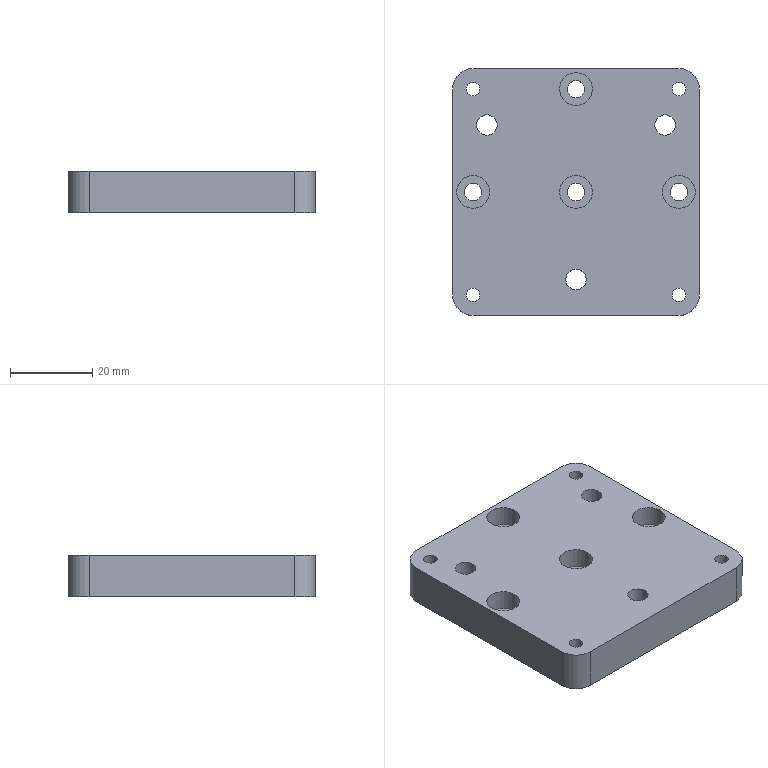Part | SolidWorks | features Cut 3, HoleWzd 3, Extrusion 1, Fillet 1, ICE 1 | 1 solid | 44 faces | box 60 x 60 x 10 mm | volume 33572 mm3 | cylinder 34 | plane 10 | commonest cylinder face diameters 3.3 x8 4.2 x8 8 x8 5 x6 10 x4
STEP:
#1=CARTESIAN_POINT('',(7.064,0.,0.));
#2=VERTEX_POINT('',#1);
#3=CARTESIAN_POINT('',(11.264,0.,0.));
#4=VERTEX_POINT('',#3);
#5=CARTESIAN_POINT('',(9.164,0.,0.));
#6=DIRECTION('',(0.,0.,1.));
#7=DIRECTION('',(1.,0.,0.));
#8=AXIS2_PLACEMENT_3D('',#5,#6,#7);
#9=CIRCLE('',#8,2.1);
#10=EDGE_CURVE('',#2,#4,#9,.T.);
#11=ORIENTED_EDGE('',*,*,#10,.F.);
#12=CARTESIAN_POINT('',(7.064,0.,5.));
#13=VERTEX_POINT('',#12);
#14=CARTESIAN_POINT('',(7.064,0.,0.));
#15=DIRECTION('',(0.,0.,1.));
#16=VECTOR('',#15,1000.);
#17=LINE('',#14,#16);
#18=EDGE_CURVE('',#2,#13,#17,.T.);
#19=ORIENTED_EDGE('',*,*,#18,.T.);
#20=CARTESIAN_POINT('',(11.264,0.,5.));
#21=VERTEX_POINT('',#20);
#22=CARTESIAN_POINT('',(9.164,0.,5.));
#23=DIRECTION('',(0.,0.,1.));
#24=DIRECTION('',(1.,0.,0.));
#25=AXIS2_PLACEMENT_3D('',#22,#23,#24);
#26=CIRCLE('',#25,2.1);
#27=EDGE_CURVE('',#13,#21,#26,.T.);
#28=ORIENTED_EDGE('',*,*,#27,.T.);
#29=CARTESIAN_POINT('',(11.264,0.,0.));
#30=DIRECTION('',(0.,0.,1.));
#31=VECTOR('',#30,1000.);
#32=LINE('',#29,#31);
#33=EDGE_CURVE('',#4,#21,#32,.T.);
#34=ORIENTED_EDGE('',*,*,#33,.F.);
#35=EDGE_LOOP('',(#11,#19,#28,#34));
#36=FACE_OUTER_BOUND('',#35,.T.);
#37=CARTESIAN_POINT('',(9.164,0.,0.));
#38=DIRECTION('',(0.,0.,1.));
#39=DIRECTION('',(1.,0.,0.));
#40=AXIS2_PLACEMENT_3D('',#37,#38,#39);
#41=CYLINDRICAL_SURFACE('',#40,2.1);
#42=ADVANCED_FACE('',(#36),#41,.F.);
#43=CARTESIAN_POINT('',(5.164,0.,5.));
#44=VERTEX_POINT('',#43);
#45=CARTESIAN_POINT('',(13.164,0.,5.));
#46=VERTEX_POINT('',#45);
#47=CARTESIAN_POINT('',(9.164,0.,5.));
#48=DIRECTION('',(0.,0.,1.));
#49=DIRECTION('',(1.,0.,0.));
#50=AXIS2_PLACEMENT_3D('',#47,#48,#49);
#51=CIRCLE('',#50,4.);
#52=EDGE_CURVE('',#44,#46,#51,.T.);
#53=ORIENTED_EDGE('',*,*,#52,.F.);
#54=CARTESIAN_POINT('',(5.164,0.,10.));
#55=VERTEX_POINT('',#54);
#56=CARTESIAN_POINT('',(5.164,0.,5.));
#57=DIRECTION('',(0.,0.,1.));
#58=VECTOR('',#57,1000.);
#59=LINE('',#56,#58);
#60=EDGE_CURVE('',#44,#55,#59,.T.);
#61=ORIENTED_EDGE('',*,*,#60,.T.);
#62=CARTESIAN_POINT('',(13.164,0.,10.));
#63=VERTEX_POINT('',#62);
#64=CARTESIAN_POINT('',(9.164,0.,10.));
#65=DIRECTION('',(0.,0.,1.));
#66=DIRECTION('',(1.,0.,0.));
#67=AXIS2_PLACEMENT_3D('',#64,#65,#66);
#68=CIRCLE('',#67,4.);
#69=EDGE_CURVE('',#55,#63,#68,.T.);
#70=ORIENTED_EDGE('',*,*,#69,.T.);
#71=CARTESIAN_POINT('',(13.164,0.,5.));
#72=DIRECTION('',(0.,0.,1.));
#73=VECTOR('',#72,1000.);
#74=LINE('',#71,#73);
#75=EDGE_CURVE('',#46,#63,#74,.T.);
#76=ORIENTED_EDGE('',*,*,#75,.F.);
#77=EDGE_LOOP('',(#53,#61,#70,#76));
#78=FACE_OUTER_BOUND('',#77,.T.);
#79=CARTESIAN_POINT('',(9.164,0.,5.));
#80=DIRECTION('',(0.,0.,1.));
#81=DIRECTION('',(1.,0.,0.));
#82=AXIS2_PLACEMENT_3D('',#79,#80,#81);
#83=CYLINDRICAL_SURFACE('',#82,4.);
#84=ADVANCED_FACE('',(#78),#83,.F.);
#85=CARTESIAN_POINT('',(-17.486,-25.,0.));
#86=VERTEX_POINT('',#85);
#87=CARTESIAN_POINT('',(-14.186,-25.,0.));
#88=VERTEX_POINT('',#87);
#89=CARTESIAN_POINT('',(-15.836,-25.,0.));
#90=DIRECTION('',(0.,0.,1.));
#91=DIRECTION('',(1.,0.,0.));
#92=AXIS2_PLACEMENT_3D('',#89,#90,#91);
#93=CIRCLE('',#92,1.65);
#94=EDGE_CURVE('',#86,#88,#93,.T.);
#95=ORIENTED_EDGE('',*,*,#94,.F.);
#96=CARTESIAN_POINT('',(-17.486,-25.,10.));
#97=VERTEX_POINT('',#96);
#98=CARTESIAN_POINT('',(-17.486,-25.,10.));
#99=DIRECTION('',(0.,0.,1.));
#100=VECTOR('',#99,1000.);
#101=LINE('',#98,#100);
#102=EDGE_CURVE('',#86,#97,#101,.T.);
#103=ORIENTED_EDGE('',*,*,#102,.T.);
#104=CARTESIAN_POINT('',(-14.186,-25.,10.));
#105=VERTEX_POINT('',#104);
#106=CARTESIAN_POINT('',(-15.836,-25.,10.));
#107=DIRECTION('',(0.,0.,1.));
#108=DIRECTION('',(1.,0.,0.));
#109=AXIS2_PLACEMENT_3D('',#106,#107,#108);
#110=CIRCLE('',#109,1.65);
#111=EDGE_CURVE('',#97,#105,#110,.T.);
#112=ORIENTED_EDGE('',*,*,#111,.T.);
#113=CARTESIAN_POINT('',(-14.186,-25.,10.));
#114=DIRECTION('',(0.,0.,1.));
#115=VECTOR('',#114,1000.);
#116=LINE('',#113,#115);
#117=EDGE_CURVE('',#88,#105,#116,.T.);
#118=ORIENTED_EDGE('',*,*,#117,.F.);
#119=EDGE_LOOP('',(#95,#103,#112,#118));
#120=FACE_OUTER_BOUND('',#119,.T.);
#121=CARTESIAN_POINT('',(-15.836,-25.,10.));
#122=DIRECTION('',(0.,0.,1.));
#123=DIRECTION('',(1.,0.,0.));
#124=AXIS2_PLACEMENT_3D('',#121,#122,#123);
#125=CYLINDRICAL_SURFACE('',#124,1.65);
#126=ADVANCED_FACE('',(#120),#125,.F.);
#127=CARTESIAN_POINT('',(32.514,-25.,0.));
#128=VERTEX_POINT('',#127);
#129=CARTESIAN_POINT('',(35.814,-25.,0.));
#130=VERTEX_POINT('',#129);
#131=CARTESIAN_POINT('',(34.164,-25.,0.));
#132=DIRECTION('',(0.,0.,1.));
#133=DIRECTION('',(1.,0.,0.));
#134=AXIS2_PLACEMENT_3D('',#131,#132,#133);
#135=CIRCLE('',#134,1.65);
#136=EDGE_CURVE('',#128,#130,#135,.T.);
#137=ORIENTED_EDGE('',*,*,#136,.F.);
#138=CARTESIAN_POINT('',(32.514,-25.,10.));
#139=VERTEX_POINT('',#138);
#140=CARTESIAN_POINT('',(32.514,-25.,10.));
#141=DIRECTION('',(0.,0.,1.));
#142=VECTOR('',#141,1000.);
#143=LINE('',#140,#142);
#144=EDGE_CURVE('',#128,#139,#143,.T.);
#145=ORIENTED_EDGE('',*,*,#144,.T.);
#146=CARTESIAN_POINT('',(35.814,-25.,10.));
#147=VERTEX_POINT('',#146);
#148=CARTESIAN_POINT('',(34.164,-25.,10.));
#149=DIRECTION('',(0.,0.,1.));
#150=DIRECTION('',(1.,0.,0.));
#151=AXIS2_PLACEMENT_3D('',#148,#149,#150);
#152=CIRCLE('',#151,1.65);
#153=EDGE_CURVE('',#139,#147,#152,.T.);
#154=ORIENTED_EDGE('',*,*,#153,.T.);
#155=CARTESIAN_POINT('',(35.814,-25.,10.));
#156=DIRECTION('',(0.,0.,1.));
#157=VECTOR('',#156,1000.);
#158=LINE('',#155,#157);
#159=EDGE_CURVE('',#130,#147,#158,.T.);
#160=ORIENTED_EDGE('',*,*,#159,.F.);
#161=EDGE_LOOP('',(#137,#145,#154,#160));
#162=FACE_OUTER_BOUND('',#161,.T.);
#163=CARTESIAN_POINT('',(34.164,-25.,10.));
#164=DIRECTION('',(0.,0.,1.));
#165=DIRECTION('',(1.,0.,0.));
#166=AXIS2_PLACEMENT_3D('',#163,#164,#165);
#167=CYLINDRICAL_SURFACE('',#166,1.65);
#168=ADVANCED_FACE('',(#162),#167,.F.);
#169=CARTESIAN_POINT('',(32.514,25.,0.));
#170=VERTEX_POINT('',#169);
#171=CARTESIAN_POINT('',(35.814,25.,0.));
#172=VERTEX_POINT('',#171);
#173=CARTESIAN_POINT('',(34.164,25.,0.));
#174=DIRECTION('',(0.,0.,1.));
#175=DIRECTION('',(1.,0.,0.));
#176=AXIS2_PLACEMENT_3D('',#173,#174,#175);
#177=CIRCLE('',#176,1.65);
#178=EDGE_CURVE('',#170,#172,#177,.T.);
#179=ORIENTED_EDGE('',*,*,#178,.F.);
#180=CARTESIAN_POINT('',(32.514,25.,10.));
#181=VERTEX_POINT('',#180);
#182=CARTESIAN_POINT('',(32.514,25.,10.));
#183=DIRECTION('',(0.,0.,1.));
#184=VECTOR('',#183,1000.);
#185=LINE('',#182,#184);
#186=EDGE_CURVE('',#170,#181,#185,.T.);
#187=ORIENTED_EDGE('',*,*,#186,.T.);
#188=CARTESIAN_POINT('',(35.814,25.,10.));
#189=VERTEX_POINT('',#188);
#190=CARTESIAN_POINT('',(34.164,25.,10.));
#191=DIRECTION('',(0.,0.,1.));
#192=DIRECTION('',(1.,0.,0.));
#193=AXIS2_PLACEMENT_3D('',#190,#191,#192);
#194=CIRCLE('',#193,1.65);
#195=EDGE_CURVE('',#181,#189,#194,.T.);
#196=ORIENTED_EDGE('',*,*,#195,.T.);
#197=CARTESIAN_POINT('',(35.814,25.,10.));
#198=DIRECTION('',(0.,0.,1.));
#199=VECTOR('',#198,1000.);
#200=LINE('',#197,#199);
#201=EDGE_CURVE('',#172,#189,#200,.T.);
#202=ORIENTED_EDGE('',*,*,#201,.F.);
#203=EDGE_LOOP('',(#179,#187,#196,#202));
#204=FACE_OUTER_BOUND('',#203,.T.);
#205=CARTESIAN_POINT('',(34.164,25.,10.));
#206=DIRECTION('',(0.,0.,1.));
#207=DIRECTION('',(1.,0.,0.));
#208=AXIS2_PLACEMENT_3D('',#205,#206,#207);
#209=CYLINDRICAL_SURFACE('',#208,1.65);
#210=ADVANCED_FACE('',(#204),#209,.F.);
#211=CARTESIAN_POINT('',(-17.486,25.,0.));
#212=VERTEX_POINT('',#211);
#213=CARTESIAN_POINT('',(-14.186,25.,0.));
#214=VERTEX_POINT('',#213);
#215=CARTESIAN_POINT('',(-15.836,25.,0.));
#216=DIRECTION('',(0.,0.,1.));
#217=DIRECTION('',(1.,0.,0.));
#218=AXIS2_PLACEMENT_3D('',#215,#216,#217);
#219=CIRCLE('',#218,1.65);
#220=EDGE_CURVE('',#212,#214,#219,.T.);
#221=ORIENTED_EDGE('',*,*,#220,.F.);
#222=CARTESIAN_POINT('',(-17.486,25.,10.));
#223=VERTEX_POINT('',#222);
#224=CARTESIAN_POINT('',(-17.486,25.,10.));
#225=DIRECTION('',(0.,0.,1.));
#226=VECTOR('',#225,1000.);
#227=LINE('',#224,#226);
#228=EDGE_CURVE('',#212,#223,#227,.T.);
#229=ORIENTED_EDGE('',*,*,#228,.T.);
#230=CARTESIAN_POINT('',(-14.186,25.,10.));
#231=VERTEX_POINT('',#230);
#232=CARTESIAN_POINT('',(-15.836,25.,10.));
#233=DIRECTION('',(0.,0.,1.));
#234=DIRECTION('',(1.,0.,0.));
#235=AXIS2_PLACEMENT_3D('',#232,#233,#234);
#236=CIRCLE('',#235,1.65);
#237=EDGE_CURVE('',#223,#231,#236,.T.);
#238=ORIENTED_EDGE('',*,*,#237,.T.);
#239=CARTESIAN_POINT('',(-14.186,25.,10.));
#240=DIRECTION('',(0.,0.,1.));
#241=VECTOR('',#240,1000.);
#242=LINE('',#239,#241);
#243=EDGE_CURVE('',#214,#231,#242,.T.);
#244=ORIENTED_EDGE('',*,*,#243,.F.);
#245=EDGE_LOOP('',(#221,#229,#238,#244));
#246=FACE_OUTER_BOUND('',#245,.T.);
#247=CARTESIAN_POINT('',(-15.836,25.,10.));
#248=DIRECTION('',(0.,0.,1.));
#249=DIRECTION('',(1.,0.,0.));
#250=AXIS2_PLACEMENT_3D('',#247,#248,#249);
#251=CYLINDRICAL_SURFACE('',#250,1.65);
#252=ADVANCED_FACE('',(#246),#251,.F.);
#253=CARTESIAN_POINT('',(-19.836,0.,5.));
#254=VERTEX_POINT('',#253);
#255=CARTESIAN_POINT('',(-11.836,0.,5.));
#256=VERTEX_POINT('',#255);
#257=CARTESIAN_POINT('',(-15.836,0.,5.));
#258=DIRECTION('',(0.,0.,1.));
#259=DIRECTION('',(1.,0.,0.));
#260=AXIS2_PLACEMENT_3D('',#257,#258,#259);
#261=CIRCLE('',#260,4.);
#262=EDGE_CURVE('',#254,#256,#261,.T.);
#263=ORIENTED_EDGE('',*,*,#262,.F.);
#264=CARTESIAN_POINT('',(-19.836,0.,10.));
#265=VERTEX_POINT('',#264);
#266=CARTESIAN_POINT('',(-19.836,0.,5.));
#267=DIRECTION('',(0.,0.,1.));
#268=VECTOR('',#267,1000.);
#269=LINE('',#266,#268);
#270=EDGE_CURVE('',#254,#265,#269,.T.);
#271=ORIENTED_EDGE('',*,*,#270,.T.);
#272=CARTESIAN_POINT('',(-11.836,0.,10.));
#273=VERTEX_POINT('',#272);
#274=CARTESIAN_POINT('',(-15.836,0.,10.));
#275=DIRECTION('',(0.,0.,1.));
#276=DIRECTION('',(1.,0.,0.));
#277=AXIS2_PLACEMENT_3D('',#274,#275,#276);
#278=CIRCLE('',#277,4.);
#279=EDGE_CURVE('',#265,#273,#278,.T.);
#280=ORIENTED_EDGE('',*,*,#279,.T.);
#281=CARTESIAN_POINT('',(-11.836,0.,5.));
#282=DIRECTION('',(0.,0.,1.));
#283=VECTOR('',#282,1000.);
#284=LINE('',#281,#283);
#285=EDGE_CURVE('',#256,#273,#284,.T.);
#286=ORIENTED_EDGE('',*,*,#285,.F.);
#287=EDGE_LOOP('',(#263,#271,#280,#286));
#288=FACE_OUTER_BOUND('',#287,.T.);
#289=CARTESIAN_POINT('',(-15.836,0.,5.));
#290=DIRECTION('',(0.,0.,1.));
#291=DIRECTION('',(1.,0.,0.));
#292=AXIS2_PLACEMENT_3D('',#289,#290,#291);
#293=CYLINDRICAL_SURFACE('',#292,4.);
#294=ADVANCED_FACE('',(#288),#293,.F.);
#295=CARTESIAN_POINT('',(30.164,0.,5.));
#296=VERTEX_POINT('',#295);
#297=CARTESIAN_POINT('',(38.164,0.,5.));
#298=VERTEX_POINT('',#297);
#299=CARTESIAN_POINT('',(34.164,0.,5.));
#300=DIRECTION('',(0.,0.,1.));
#301=DIRECTION('',(1.,0.,0.));
#302=AXIS2_PLACEMENT_3D('',#299,#300,#301);
#303=CIRCLE('',#302,4.);
#304=EDGE_CURVE('',#296,#298,#303,.T.);
#305=ORIENTED_EDGE('',*,*,#304,.F.);
#306=CARTESIAN_POINT('',(30.164,0.,10.));
#307=VERTEX_POINT('',#306);
#308=CARTESIAN_POINT('',(30.164,0.,5.));
#309=DIRECTION('',(0.,0.,1.));
#310=VECTOR('',#309,1000.);
#311=LINE('',#308,#310);
#312=EDGE_CURVE('',#296,#307,#311,.T.);
#313=ORIENTED_EDGE('',*,*,#312,.T.);
#314=CARTESIAN_POINT('',(38.164,0.,10.));
#315=VERTEX_POINT('',#314);
#316=CARTESIAN_POINT('',(34.164,0.,10.));
#317=DIRECTION('',(0.,0.,1.));
#318=DIRECTION('',(1.,0.,0.));
#319=AXIS2_PLACEMENT_3D('',#316,#317,#318);
#320=CIRCLE('',#319,4.);
#321=EDGE_CURVE('',#307,#315,#320,.T.);
#322=ORIENTED_EDGE('',*,*,#321,.T.);
#323=CARTESIAN_POINT('',(38.164,0.,5.));
#324=DIRECTION('',(0.,0.,1.));
#325=VECTOR('',#324,1000.);
#326=LINE('',#323,#325);
#327=EDGE_CURVE('',#298,#315,#326,.T.);
#328=ORIENTED_EDGE('',*,*,#327,.F.);
#329=EDGE_LOOP('',(#305,#313,#322,#328));
#330=FACE_OUTER_BOUND('',#329,.T.);
#331=CARTESIAN_POINT('',(34.164,0.,5.));
#332=DIRECTION('',(0.,0.,1.));
#333=DIRECTION('',(1.,0.,0.));
#334=AXIS2_PLACEMENT_3D('',#331,#332,#333);
#335=CYLINDRICAL_SURFACE('',#334,4.);
#336=ADVANCED_FACE('',(#330),#335,.F.);
#337=CARTESIAN_POINT('',(5.164,25.,5.));
#338=VERTEX_POINT('',#337);
#339=CARTESIAN_POINT('',(13.164,25.,5.));
#340=VERTEX_POINT('',#339);
#341=CARTESIAN_POINT('',(9.164,25.,5.));
#342=DIRECTION('',(0.,0.,1.));
#343=DIRECTION('',(1.,0.,0.));
#344=AXIS2_PLACEMENT_3D('',#341,#342,#343);
#345=CIRCLE('',#344,4.);
#346=EDGE_CURVE('',#338,#340,#345,.T.);
#347=ORIENTED_EDGE('',*,*,#346,.F.);
#348=CARTESIAN_POINT('',(5.164,25.,10.));
#349=VERTEX_POINT('',#348);
#350=CARTESIAN_POINT('',(5.164,25.,5.));
#351=DIRECTION('',(0.,0.,1.));
#352=VECTOR('',#351,1000.);
#353=LINE('',#350,#352);
#354=EDGE_CURVE('',#338,#349,#353,.T.);
#355=ORIENTED_EDGE('',*,*,#354,.T.);
#356=CARTESIAN_POINT('',(13.164,25.,10.));
#357=VERTEX_POINT('',#356);
#358=CARTESIAN_POINT('',(9.164,25.,10.));
#359=DIRECTION('',(0.,0.,1.));
#360=DIRECTION('',(1.,0.,0.));
#361=AXIS2_PLACEMENT_3D('',#358,#359,#360);
#362=CIRCLE('',#361,4.);
#363=EDGE_CURVE('',#349,#357,#362,.T.);
#364=ORIENTED_EDGE('',*,*,#363,.T.);
#365=CARTESIAN_POINT('',(13.164,25.,5.));
#366=DIRECTION('',(0.,0.,1.));
#367=VECTOR('',#366,1000.);
#368=LINE('',#365,#367);
#369=EDGE_CURVE('',#340,#357,#368,.T.);
#370=ORIENTED_EDGE('',*,*,#369,.F.);
#371=EDGE_LOOP('',(#347,#355,#364,#370));
#372=FACE_OUTER_BOUND('',#371,.T.);
#373=CARTESIAN_POINT('',(9.164,25.,5.));
#374=DIRECTION('',(0.,0.,1.));
#375=DIRECTION('',(1.,0.,0.));
#376=AXIS2_PLACEMENT_3D('',#373,#374,#375);
#377=CYLINDRICAL_SURFACE('',#376,4.);
#378=ADVANCED_FACE('',(#372),#377,.F.);
#379=CARTESIAN_POINT('',(6.664,-21.25,0.));
#380=VERTEX_POINT('',#379);
#381=CARTESIAN_POINT('',(11.664,-21.25,0.));
#382=VERTEX_POINT('',#381);
#383=CARTESIAN_POINT('',(9.164,-21.25,0.));
#384=DIRECTION('',(0.,0.,1.));
#385=DIRECTION('',(1.,0.,0.));
#386=AXIS2_PLACEMENT_3D('',#383,#384,#385);
#387=CIRCLE('',#386,2.5);
#388=EDGE_CURVE('',#380,#382,#387,.T.);
#389=ORIENTED_EDGE('',*,*,#388,.F.);
#390=CARTESIAN_POINT('',(6.664,-21.25,10.));
#391=VERTEX_POINT('',#390);
#392=CARTESIAN_POINT('',(6.664,-21.25,10.));
#393=DIRECTION('',(0.,0.,1.));
#394=VECTOR('',#393,1000.);
#395=LINE('',#392,#394);
#396=EDGE_CURVE('',#380,#391,#395,.T.);
#397=ORIENTED_EDGE('',*,*,#396,.T.);
#398=CARTESIAN_POINT('',(11.664,-21.25,10.));
#399=VERTEX_POINT('',#398);
#400=CARTESIAN_POINT('',(9.164,-21.25,10.));
#401=DIRECTION('',(0.,0.,1.));
#402=DIRECTION('',(1.,0.,0.));
#403=AXIS2_PLACEMENT_3D('',#400,#401,#402);
#404=CIRCLE('',#403,2.5);
#405=EDGE_CURVE('',#391,#399,#404,.T.);
#406=ORIENTED_EDGE('',*,*,#405,.T.);
#407=CARTESIAN_POINT('',(11.664,-21.25,10.));
#408=DIRECTION('',(0.,0.,1.));
#409=VECTOR('',#408,1000.);
#410=LINE('',#407,#409);
#411=EDGE_CURVE('',#382,#399,#410,.T.);
#412=ORIENTED_EDGE('',*,*,#411,.F.);
#413=EDGE_LOOP('',(#389,#397,#406,#412));
#414=FACE_OUTER_BOUND('',#413,.T.);
#415=CARTESIAN_POINT('',(9.164,-21.25,10.));
#416=DIRECTION('',(0.,0.,1.));
#417=DIRECTION('',(1.,0.,0.));
#418=AXIS2_PLACEMENT_3D('',#415,#416,#417);
#419=CYLINDRICAL_SURFACE('',#418,2.5);
#420=ADVANCED_FACE('',(#414),#419,.F.);
#421=CARTESIAN_POINT('',(28.314,16.25,0.));
#422=VERTEX_POINT('',#421);
#423=CARTESIAN_POINT('',(33.314,16.25,0.));
#424=VERTEX_POINT('',#423);
#425=CARTESIAN_POINT('',(30.814,16.25,0.));
#426=DIRECTION('',(0.,0.,1.));
#427=DIRECTION('',(1.,0.,0.));
#428=AXIS2_PLACEMENT_3D('',#425,#426,#427);
#429=CIRCLE('',#428,2.5);
#430=EDGE_CURVE('',#422,#424,#429,.T.);
#431=ORIENTED_EDGE('',*,*,#430,.F.);
#432=CARTESIAN_POINT('',(28.314,16.25,10.));
#433=VERTEX_POINT('',#432);
#434=CARTESIAN_POINT('',(28.314,16.25,10.));
#435=DIRECTION('',(0.,0.,1.));
#436=VECTOR('',#435,1000.);
#437=LINE('',#434,#436);
#438=EDGE_CURVE('',#422,#433,#437,.T.);
#439=ORIENTED_EDGE('',*,*,#438,.T.);
#440=CARTESIAN_POINT('',(33.314,16.25,10.));
#441=VERTEX_POINT('',#440);
#442=CARTESIAN_POINT('',(30.814,16.25,10.));
#443=DIRECTION('',(0.,0.,1.));
#444=DIRECTION('',(1.,0.,0.));
#445=AXIS2_PLACEMENT_3D('',#442,#443,#444);
#446=CIRCLE('',#445,2.5);
#447=EDGE_CURVE('',#433,#441,#446,.T.);
#448=ORIENTED_EDGE('',*,*,#447,.T.);
#449=CARTESIAN_POINT('',(33.314,16.25,10.));
#450=DIRECTION('',(0.,0.,1.));
#451=VECTOR('',#450,1000.);
#452=LINE('',#449,#451);
#453=EDGE_CURVE('',#424,#441,#452,.T.);
#454=ORIENTED_EDGE('',*,*,#453,.F.);
#455=EDGE_LOOP('',(#431,#439,#448,#454));
#456=FACE_OUTER_BOUND('',#455,.T.);
#457=CARTESIAN_POINT('',(30.814,16.25,10.));
#458=DIRECTION('',(0.,0.,1.));
#459=DIRECTION('',(1.,0.,0.));
#460=AXIS2_PLACEMENT_3D('',#457,#458,#459);
#461=CYLINDRICAL_SURFACE('',#460,2.5);
#462=ADVANCED_FACE('',(#456),#461,.F.);
#463=CARTESIAN_POINT('',(-14.987,16.25,0.));
#464=VERTEX_POINT('',#463);
#465=CARTESIAN_POINT('',(-9.987,16.25,0.));
#466=VERTEX_POINT('',#465);
#467=CARTESIAN_POINT('',(-12.487,16.25,0.));
#468=DIRECTION('',(0.,0.,1.));
#469=DIRECTION('',(1.,0.,0.));
#470=AXIS2_PLACEMENT_3D('',#467,#468,#469);
#471=CIRCLE('',#470,2.5);
#472=EDGE_CURVE('',#464,#466,#471,.T.);
#473=ORIENTED_EDGE('',*,*,#472,.F.);
#474=CARTESIAN_POINT('',(-14.987,16.25,10.));
#475=VERTEX_POINT('',#474);
#476=CARTESIAN_POINT('',(-14.987,16.25,10.));
#477=DIRECTION('',(0.,0.,1.));
#478=VECTOR('',#477,1000.);
#479=LINE('',#476,#478);
#480=EDGE_CURVE('',#464,#475,#479,.T.);
#481=ORIENTED_EDGE('',*,*,#480,.T.);
#482=CARTESIAN_POINT('',(-9.987,16.25,10.));
#483=VERTEX_POINT('',#482);
#484=CARTESIAN_POINT('',(-12.487,16.25,10.));
#485=DIRECTION('',(0.,0.,1.));
#486=DIRECTION('',(1.,0.,0.));
#487=AXIS2_PLACEMENT_3D('',#484,#485,#486);
#488=CIRCLE('',#487,2.5);
#489=EDGE_CURVE('',#475,#483,#488,.T.);
#490=ORIENTED_EDGE('',*,*,#489,.T.);
#491=CARTESIAN_POINT('',(-9.987,16.25,10.));
#492=DIRECTION('',(0.,0.,1.));
#493=VECTOR('',#492,1000.);
#494=LINE('',#491,#493);
#495=EDGE_CURVE('',#466,#483,#494,.T.);
#496=ORIENTED_EDGE('',*,*,#495,.F.);
#497=EDGE_LOOP('',(#473,#481,#490,#496));
#498=FACE_OUTER_BOUND('',#497,.T.);
#499=CARTESIAN_POINT('',(-12.487,16.25,10.));
#500=DIRECTION('',(0.,0.,1.));
#501=DIRECTION('',(1.,0.,0.));
#502=AXIS2_PLACEMENT_3D('',#499,#500,#501);
#503=CYLINDRICAL_SURFACE('',#502,2.5);
#504=ADVANCED_FACE('',(#498),#503,.F.);
#505=CARTESIAN_POINT('',(7.064,25.,0.));
#506=VERTEX_POINT('',#505);
#507=CARTESIAN_POINT('',(11.264,25.,0.));
#508=VERTEX_POINT('',#507);
#509=CARTESIAN_POINT('',(9.164,25.,0.));
#510=DIRECTION('',(0.,0.,1.));
#511=DIRECTION('',(1.,0.,0.));
#512=AXIS2_PLACEMENT_3D('',#509,#510,#511);
#513=CIRCLE('',#512,2.1);
#514=EDGE_CURVE('',#506,#508,#513,.T.);
#515=ORIENTED_EDGE('',*,*,#514,.F.);
#516=CARTESIAN_POINT('',(7.064,25.,5.));
#517=VERTEX_POINT('',#516);
#518=CARTESIAN_POINT('',(7.064,25.,0.));
#519=DIRECTION('',(0.,0.,1.));
#520=VECTOR('',#519,1000.);
#521=LINE('',#518,#520);
#522=EDGE_CURVE('',#506,#517,#521,.T.);
#523=ORIENTED_EDGE('',*,*,#522,.T.);
#524=CARTESIAN_POINT('',(11.264,25.,5.));
#525=VERTEX_POINT('',#524);
#526=CARTESIAN_POINT('',(9.164,25.,5.));
#527=DIRECTION('',(0.,0.,-1.));
#528=DIRECTION('',(1.,0.,0.));
#529=AXIS2_PLACEMENT_3D('',#526,#527,#528);
#530=CIRCLE('',#529,2.1);
#531=EDGE_CURVE('',#525,#517,#530,.T.);
#532=ORIENTED_EDGE('',*,*,#531,.F.);
#533=CARTESIAN_POINT('',(11.264,25.,0.));
#534=DIRECTION('',(0.,0.,1.));
#535=VECTOR('',#534,1000.);
#536=LINE('',#533,#535);
#537=EDGE_CURVE('',#508,#525,#536,.T.);
#538=ORIENTED_EDGE('',*,*,#537,.F.);
#539=EDGE_LOOP('',(#515,#523,#532,#538));
#540=FACE_OUTER_BOUND('',#539,.T.);
#541=CARTESIAN_POINT('',(9.164,25.,0.));
#542=DIRECTION('',(0.,0.,1.));
#543=DIRECTION('',(1.,0.,0.));
#544=AXIS2_PLACEMENT_3D('',#541,#542,#543);
#545=CYLINDRICAL_SURFACE('',#544,2.1);
#546=ADVANCED_FACE('',(#540),#545,.F.);
#547=CARTESIAN_POINT('',(32.064,0.,0.));
#548=VERTEX_POINT('',#547);
#549=CARTESIAN_POINT('',(36.264,0.,0.));
#550=VERTEX_POINT('',#549);
#551=CARTESIAN_POINT('',(34.164,0.,0.));
#552=DIRECTION('',(0.,0.,1.));
#553=DIRECTION('',(1.,0.,0.));
#554=AXIS2_PLACEMENT_3D('',#551,#552,#553);
#555=CIRCLE('',#554,2.1);
#556=EDGE_CURVE('',#548,#550,#555,.T.);
#557=ORIENTED_EDGE('',*,*,#556,.F.);
#558=CARTESIAN_POINT('',(32.064,0.,5.));
#559=VERTEX_POINT('',#558);
#560=CARTESIAN_POINT('',(32.064,0.,0.));
#561=DIRECTION('',(0.,0.,1.));
#562=VECTOR('',#561,1000.);
#563=LINE('',#560,#562);
#564=EDGE_CURVE('',#548,#559,#563,.T.);
#565=ORIENTED_EDGE('',*,*,#564,.T.);
#566=CARTESIAN_POINT('',(36.264,0.,5.));
#567=VERTEX_POINT('',#566);
#568=CARTESIAN_POINT('',(34.164,0.,5.));
#569=DIRECTION('',(0.,0.,-1.));
#570=DIRECTION('',(1.,0.,0.));
#571=AXIS2_PLACEMENT_3D('',#568,#569,#570);
#572=CIRCLE('',#571,2.1);
#573=EDGE_CURVE('',#567,#559,#572,.T.);
#574=ORIENTED_EDGE('',*,*,#573,.F.);
#575=CARTESIAN_POINT('',(36.264,0.,0.));
#576=DIRECTION('',(0.,0.,1.));
#577=VECTOR('',#576,1000.);
#578=LINE('',#575,#577);
#579=EDGE_CURVE('',#550,#567,#578,.T.);
#580=ORIENTED_EDGE('',*,*,#579,.F.);
#581=EDGE_LOOP('',(#557,#565,#574,#580));
#582=FACE_OUTER_BOUND('',#581,.T.);
#583=CARTESIAN_POINT('',(34.164,0.,0.));
#584=DIRECTION('',(0.,0.,1.));
#585=DIRECTION('',(1.,0.,0.));
#586=AXIS2_PLACEMENT_3D('',#583,#584,#585);
#587=CYLINDRICAL_SURFACE('',#586,2.1);
#588=ADVANCED_FACE('',(#582),#587,.F.);
#589=CARTESIAN_POINT('',(-17.936,0.,0.));
#590=VERTEX_POINT('',#589);
#591=CARTESIAN_POINT('',(-13.736,0.,0.));
#592=VERTEX_POINT('',#591);
#593=CARTESIAN_POINT('',(-15.836,0.,0.));
#594=DIRECTION('',(0.,0.,1.));
#595=DIRECTION('',(1.,0.,0.));
#596=AXIS2_PLACEMENT_3D('',#593,#594,#595);
#597=CIRCLE('',#596,2.1);
#598=EDGE_CURVE('',#590,#592,#597,.T.);
#599=ORIENTED_EDGE('',*,*,#598,.F.);
#600=CARTESIAN_POINT('',(-17.936,0.,5.));
#601=VERTEX_POINT('',#600);
#602=CARTESIAN_POINT('',(-17.936,0.,0.));
#603=DIRECTION('',(0.,0.,1.));
#604=VECTOR('',#603,1000.);
#605=LINE('',#602,#604);
#606=EDGE_CURVE('',#590,#601,#605,.T.);
#607=ORIENTED_EDGE('',*,*,#606,.T.);
#608=CARTESIAN_POINT('',(-13.736,0.,5.));
#609=VERTEX_POINT('',#608);
#610=CARTESIAN_POINT('',(-15.836,0.,5.));
#611=DIRECTION('',(0.,0.,-1.));
#612=DIRECTION('',(1.,0.,0.));
#613=AXIS2_PLACEMENT_3D('',#610,#611,#612);
#614=CIRCLE('',#613,2.1);
#615=EDGE_CURVE('',#609,#601,#614,.T.);
#616=ORIENTED_EDGE('',*,*,#615,.F.);
#617=CARTESIAN_POINT('',(-13.736,0.,0.));
#618=DIRECTION('',(0.,0.,1.));
#619=VECTOR('',#618,1000.);
#620=LINE('',#617,#619);
#621=EDGE_CURVE('',#592,#609,#620,.T.);
#622=ORIENTED_EDGE('',*,*,#621,.F.);
#623=EDGE_LOOP('',(#599,#607,#616,#622));
#624=FACE_OUTER_BOUND('',#623,.T.);
#625=CARTESIAN_POINT('',(-15.836,0.,0.));
#626=DIRECTION('',(0.,0.,1.));
#627=DIRECTION('',(1.,0.,0.));
#628=AXIS2_PLACEMENT_3D('',#625,#626,#627);
#629=CYLINDRICAL_SURFACE('',#628,2.1);
#630=ADVANCED_FACE('',(#624),#629,.F.);
#631=ORIENTED_EDGE('',*,*,#606,.F.);
#632=CARTESIAN_POINT('',(-15.836,0.,0.));
#633=DIRECTION('',(0.,0.,1.));
#634=DIRECTION('',(1.,0.,0.));
#635=AXIS2_PLACEMENT_3D('',#632,#633,#634);
#636=CIRCLE('',#635,2.1);
#637=EDGE_CURVE('',#592,#590,#636,.T.);
#638=ORIENTED_EDGE('',*,*,#637,.F.);
#639=ORIENTED_EDGE('',*,*,#621,.T.);
#640=CARTESIAN_POINT('',(-15.836,0.,5.));
#641=DIRECTION('',(0.,0.,-1.));
#642=DIRECTION('',(1.,0.,0.));
#643=AXIS2_PLACEMENT_3D('',#640,#641,#642);
#644=CIRCLE('',#643,2.1);
#645=EDGE_CURVE('',#601,#609,#644,.T.);
#646=ORIENTED_EDGE('',*,*,#645,.F.);
#647=EDGE_LOOP('',(#631,#638,#639,#646));
#648=FACE_OUTER_BOUND('',#647,.T.);
#649=CARTESIAN_POINT('',(-15.836,0.,0.));
#650=DIRECTION('',(0.,0.,1.));
#651=DIRECTION('',(1.,0.,0.));
#652=AXIS2_PLACEMENT_3D('',#649,#650,#651);
#653=CYLINDRICAL_SURFACE('',#652,2.1);
#654=ADVANCED_FACE('',(#648),#653,.F.);
#655=ORIENTED_EDGE('',*,*,#564,.F.);
#656=CARTESIAN_POINT('',(34.164,0.,0.));
#657=DIRECTION('',(0.,0.,1.));
#658=DIRECTION('',(1.,0.,0.));
#659=AXIS2_PLACEMENT_3D('',#656,#657,#658);
#660=CIRCLE('',#659,2.1);
#661=EDGE_CURVE('',#550,#548,#660,.T.);
#662=ORIENTED_EDGE('',*,*,#661,.F.);
#663=ORIENTED_EDGE('',*,*,#579,.T.);
#664=CARTESIAN_POINT('',(34.164,0.,5.));
#665=DIRECTION('',(0.,0.,-1.));
#666=DIRECTION('',(1.,0.,0.));
#667=AXIS2_PLACEMENT_3D('',#664,#665,#666);
#668=CIRCLE('',#667,2.1);
#669=EDGE_CURVE('',#559,#567,#668,.T.);
#670=ORIENTED_EDGE('',*,*,#669,.F.);
#671=EDGE_LOOP('',(#655,#662,#663,#670));
#672=FACE_OUTER_BOUND('',#671,.T.);
#673=CARTESIAN_POINT('',(34.164,0.,0.));
#674=DIRECTION('',(0.,0.,1.));
#675=DIRECTION('',(1.,0.,0.));
#676=AXIS2_PLACEMENT_3D('',#673,#674,#675);
#677=CYLINDRICAL_SURFACE('',#676,2.1);
#678=ADVANCED_FACE('',(#672),#677,.F.);
#679=ORIENTED_EDGE('',*,*,#522,.F.);
#680=CARTESIAN_POINT('',(9.164,25.,0.));
#681=DIRECTION('',(0.,0.,1.));
#682=DIRECTION('',(1.,0.,0.));
#683=AXIS2_PLACEMENT_3D('',#680,#681,#682);
#684=CIRCLE('',#683,2.1);
#685=EDGE_CURVE('',#508,#506,#684,.T.);
#686=ORIENTED_EDGE('',*,*,#685,.F.);
#687=ORIENTED_EDGE('',*,*,#537,.T.);
#688=CARTESIAN_POINT('',(9.164,25.,5.));
#689=DIRECTION('',(0.,0.,-1.));
#690=DIRECTION('',(1.,0.,0.));
#691=AXIS2_PLACEMENT_3D('',#688,#689,#690);
#692=CIRCLE('',#691,2.1);
#693=EDGE_CURVE('',#517,#525,#692,.T.);
#694=ORIENTED_EDGE('',*,*,#693,.F.);
#695=EDGE_LOOP('',(#679,#686,#687,#694));
#696=FACE_OUTER_BOUND('',#695,.T.);
#697=CARTESIAN_POINT('',(9.164,25.,0.));
#698=DIRECTION('',(0.,0.,1.));
#699=DIRECTION('',(1.,0.,0.));
#700=AXIS2_PLACEMENT_3D('',#697,#698,#699);
#701=CYLINDRICAL_SURFACE('',#700,2.1);
#702=ADVANCED_FACE('',(#696),#701,.F.);
#703=CARTESIAN_POINT('',(-20.836,25.,10.));
#704=VERTEX_POINT('',#703);
#705=CARTESIAN_POINT('',(-20.836,-25.,10.));
#706=VERTEX_POINT('',#705);
#707=CARTESIAN_POINT('',(-20.836,-30.,10.));
#708=DIRECTION('',(0.,-1.,0.));
#709=VECTOR('',#708,1000.);
#710=LINE('',#707,#709);
#711=EDGE_CURVE('',#704,#706,#710,.T.);
#712=ORIENTED_EDGE('',*,*,#711,.F.);
#713=CARTESIAN_POINT('',(-20.836,25.,0.));
#714=VERTEX_POINT('',#713);
#715=CARTESIAN_POINT('',(-20.836,25.,10.));
#716=DIRECTION('',(0.,0.,-1.));
#717=VECTOR('',#716,1000.);
#718=LINE('',#715,#717);
#719=EDGE_CURVE('',#704,#714,#718,.T.);
#720=ORIENTED_EDGE('',*,*,#719,.T.);
#721=CARTESIAN_POINT('',(-20.836,-25.,0.));
#722=VERTEX_POINT('',#721);
#723=CARTESIAN_POINT('',(-20.836,-30.,0.));
#724=DIRECTION('',(0.,-1.,0.));
#725=VECTOR('',#724,1000.);
#726=LINE('',#723,#725);
#727=EDGE_CURVE('',#714,#722,#726,.T.);
#728=ORIENTED_EDGE('',*,*,#727,.T.);
#729=CARTESIAN_POINT('',(-20.836,-25.,10.));
#730=DIRECTION('',(0.,0.,1.));
#731=VECTOR('',#730,1000.);
#732=LINE('',#729,#731);
#733=EDGE_CURVE('',#722,#706,#732,.T.);
#734=ORIENTED_EDGE('',*,*,#733,.T.);
#735=EDGE_LOOP('',(#712,#720,#728,#734));
#736=FACE_OUTER_BOUND('',#735,.T.);
#737=CARTESIAN_POINT('',(-20.836,-30.,10.));
#738=DIRECTION('',(1.,0.,0.));
#739=DIRECTION('',(0.,0.,-1.));
#740=AXIS2_PLACEMENT_3D('',#737,#738,#739);
#741=PLANE('',#740);
#742=ADVANCED_FACE('',(#736),#741,.F.);
#743=CARTESIAN_POINT('',(-15.836,-30.,0.));
#744=VERTEX_POINT('',#743);
#745=CARTESIAN_POINT('',(34.164,-30.,0.));
#746=VERTEX_POINT('',#745);
#747=CARTESIAN_POINT('',(39.164,-30.,0.));
#748=DIRECTION('',(1.,0.,0.));
#749=VECTOR('',#748,1000.);
#750=LINE('',#747,#749);
#751=EDGE_CURVE('',#744,#746,#750,.T.);
#752=ORIENTED_EDGE('',*,*,#751,.T.);
#753=CARTESIAN_POINT('',(34.164,-30.,10.));
#754=VERTEX_POINT('',#753);
#755=CARTESIAN_POINT('',(34.164,-30.,10.));
#756=DIRECTION('',(0.,0.,1.));
#757=VECTOR('',#756,1000.);
#758=LINE('',#755,#757);
#759=EDGE_CURVE('',#746,#754,#758,.T.);
#760=ORIENTED_EDGE('',*,*,#759,.T.);
#761=CARTESIAN_POINT('',(-15.836,-30.,10.));
#762=VERTEX_POINT('',#761);
#763=CARTESIAN_POINT('',(39.164,-30.,10.));
#764=DIRECTION('',(1.,0.,0.));
#765=VECTOR('',#764,1000.);
#766=LINE('',#763,#765);
#767=EDGE_CURVE('',#762,#754,#766,.T.);
#768=ORIENTED_EDGE('',*,*,#767,.F.);
#769=CARTESIAN_POINT('',(-15.836,-30.,10.));
#770=DIRECTION('',(0.,0.,-1.));
#771=VECTOR('',#770,1000.);
#772=LINE('',#769,#771);
#773=EDGE_CURVE('',#762,#744,#772,.T.);
#774=ORIENTED_EDGE('',*,*,#773,.T.);
#775=EDGE_LOOP('',(#752,#760,#768,#774));
#776=FACE_OUTER_BOUND('',#775,.T.);
#777=CARTESIAN_POINT('',(39.164,-30.,10.));
#778=DIRECTION('',(0.,1.,0.));
#779=DIRECTION('',(-1.,0.,0.));
#780=AXIS2_PLACEMENT_3D('',#777,#778,#779);
#781=PLANE('',#780);
#782=ADVANCED_FACE('',(#776),#781,.F.);
#783=CARTESIAN_POINT('',(39.164,-25.,0.));
#784=VERTEX_POINT('',#783);
#785=CARTESIAN_POINT('',(39.164,25.,0.));
#786=VERTEX_POINT('',#785);
#787=CARTESIAN_POINT('',(39.164,-30.,0.));
#788=DIRECTION('',(0.,1.,0.));
#789=VECTOR('',#788,1000.);
#790=LINE('',#787,#789);
#791=EDGE_CURVE('',#784,#786,#790,.T.);
#792=ORIENTED_EDGE('',*,*,#791,.T.);
#793=CARTESIAN_POINT('',(39.164,25.,10.));
#794=VERTEX_POINT('',#793);
#795=CARTESIAN_POINT('',(39.164,25.,10.));
#796=DIRECTION('',(0.,0.,1.));
#797=VECTOR('',#796,1000.);
#798=LINE('',#795,#797);
#799=EDGE_CURVE('',#786,#794,#798,.T.);
#800=ORIENTED_EDGE('',*,*,#799,.T.);
#801=CARTESIAN_POINT('',(39.164,-25.,10.));
#802=VERTEX_POINT('',#801);
#803=CARTESIAN_POINT('',(39.164,-30.,10.));
#804=DIRECTION('',(0.,1.,0.));
#805=VECTOR('',#804,1000.);
#806=LINE('',#803,#805);
#807=EDGE_CURVE('',#802,#794,#806,.T.);
#808=ORIENTED_EDGE('',*,*,#807,.F.);
#809=CARTESIAN_POINT('',(39.164,-25.,10.));
#810=DIRECTION('',(0.,0.,-1.));
#811=VECTOR('',#810,1000.);
#812=LINE('',#809,#811);
#813=EDGE_CURVE('',#802,#784,#812,.T.);
#814=ORIENTED_EDGE('',*,*,#813,.T.);
#815=EDGE_LOOP('',(#792,#800,#808,#814));
#816=FACE_OUTER_BOUND('',#815,.T.);
#817=CARTESIAN_POINT('',(39.164,-30.,10.));
#818=DIRECTION('',(-1.,0.,0.));
#819=DIRECTION('',(0.,0.,1.));
#820=AXIS2_PLACEMENT_3D('',#817,#818,#819);
#821=PLANE('',#820);
#822=ADVANCED_FACE('',(#816),#821,.F.);
#823=CARTESIAN_POINT('',(34.164,30.,0.));
#824=VERTEX_POINT('',#823);
#825=CARTESIAN_POINT('',(-15.836,30.,0.));
#826=VERTEX_POINT('',#825);
#827=CARTESIAN_POINT('',(39.164,30.,0.));
#828=DIRECTION('',(-1.,0.,0.));
#829=VECTOR('',#828,1000.);
#830=LINE('',#827,#829);
#831=EDGE_CURVE('',#824,#826,#830,.T.);
#832=ORIENTED_EDGE('',*,*,#831,.T.);
#833=CARTESIAN_POINT('',(-15.836,30.,10.));
#834=VERTEX_POINT('',#833);
#835=CARTESIAN_POINT('',(-15.836,30.,10.));
#836=DIRECTION('',(0.,0.,1.));
#837=VECTOR('',#836,1000.);
#838=LINE('',#835,#837);
#839=EDGE_CURVE('',#826,#834,#838,.T.);
#840=ORIENTED_EDGE('',*,*,#839,.T.);
#841=CARTESIAN_POINT('',(34.164,30.,10.));
#842=VERTEX_POINT('',#841);
#843=CARTESIAN_POINT('',(39.164,30.,10.));
#844=DIRECTION('',(-1.,0.,0.));
#845=VECTOR('',#844,1000.);
#846=LINE('',#843,#845);
#847=EDGE_CURVE('',#842,#834,#846,.T.);
#848=ORIENTED_EDGE('',*,*,#847,.F.);
#849=CARTESIAN_POINT('',(34.164,30.,10.));
#850=DIRECTION('',(0.,0.,-1.));
#851=VECTOR('',#850,1000.);
#852=LINE('',#849,#851);
#853=EDGE_CURVE('',#842,#824,#852,.T.);
#854=ORIENTED_EDGE('',*,*,#853,.T.);
#855=EDGE_LOOP('',(#832,#840,#848,#854));
#856=FACE_OUTER_BOUND('',#855,.T.);
#857=CARTESIAN_POINT('',(39.164,30.,10.));
#858=DIRECTION('',(0.,-1.,0.));
#859=DIRECTION('',(1.,0.,0.));
#860=AXIS2_PLACEMENT_3D('',#857,#858,#859);
#861=PLANE('',#860);
#862=ADVANCED_FACE('',(#856),#861,.F.);
#863=CARTESIAN_POINT('',(9.164,0.,10.));
#864=DIRECTION('',(0.,0.,1.));
#865=DIRECTION('',(1.,0.,0.));
#866=AXIS2_PLACEMENT_3D('',#863,#864,#865);
#867=CIRCLE('',#866,4.);
#868=EDGE_CURVE('',#63,#55,#867,.T.);
#869=ORIENTED_EDGE('',*,*,#868,.F.);
#870=ORIENTED_EDGE('',*,*,#69,.F.);
#871=EDGE_LOOP('',(#869,#870));
#872=FACE_BOUND('',#871,.T.);
#873=CARTESIAN_POINT('',(-15.836,-25.,10.));
#874=DIRECTION('',(0.,0.,1.));
#875=DIRECTION('',(1.,0.,0.));
#876=AXIS2_PLACEMENT_3D('',#873,#874,#875);
#877=CIRCLE('',#876,1.65);
#878=EDGE_CURVE('',#105,#97,#877,.T.);
#879=ORIENTED_EDGE('',*,*,#878,.F.);
#880=ORIENTED_EDGE('',*,*,#111,.F.);
#881=EDGE_LOOP('',(#879,#880));
#882=FACE_BOUND('',#881,.T.);
#883=CARTESIAN_POINT('',(34.164,-25.,10.));
#884=DIRECTION('',(0.,0.,1.));
#885=DIRECTION('',(1.,0.,0.));
#886=AXIS2_PLACEMENT_3D('',#883,#884,#885);
#887=CIRCLE('',#886,1.65);
#888=EDGE_CURVE('',#147,#139,#887,.T.);
#889=ORIENTED_EDGE('',*,*,#888,.F.);
#890=ORIENTED_EDGE('',*,*,#153,.F.);
#891=EDGE_LOOP('',(#889,#890));
#892=FACE_BOUND('',#891,.T.);
#893=CARTESIAN_POINT('',(34.164,25.,10.));
#894=DIRECTION('',(0.,0.,1.));
#895=DIRECTION('',(1.,0.,0.));
#896=AXIS2_PLACEMENT_3D('',#893,#894,#895);
#897=CIRCLE('',#896,1.65);
#898=EDGE_CURVE('',#189,#181,#897,.T.);
#899=ORIENTED_EDGE('',*,*,#898,.F.);
#900=ORIENTED_EDGE('',*,*,#195,.F.);
#901=EDGE_LOOP('',(#899,#900));
#902=FACE_BOUND('',#901,.T.);
#903=CARTESIAN_POINT('',(-15.836,25.,10.));
#904=DIRECTION('',(0.,0.,1.));
#905=DIRECTION('',(1.,0.,0.));
#906=AXIS2_PLACEMENT_3D('',#903,#904,#905);
#907=CIRCLE('',#906,1.65);
#908=EDGE_CURVE('',#231,#223,#907,.T.);
#909=ORIENTED_EDGE('',*,*,#908,.F.);
#910=ORIENTED_EDGE('',*,*,#237,.F.);
#911=EDGE_LOOP('',(#909,#910));
#912=FACE_BOUND('',#911,.T.);
#913=CARTESIAN_POINT('',(-15.836,0.,10.));
#914=DIRECTION('',(0.,0.,1.));
#915=DIRECTION('',(1.,0.,0.));
#916=AXIS2_PLACEMENT_3D('',#913,#914,#915);
#917=CIRCLE('',#916,4.);
#918=EDGE_CURVE('',#273,#265,#917,.T.);
#919=ORIENTED_EDGE('',*,*,#918,.F.);
#920=ORIENTED_EDGE('',*,*,#279,.F.);
#921=EDGE_LOOP('',(#919,#920));
#922=FACE_BOUND('',#921,.T.);
#923=CARTESIAN_POINT('',(9.164,25.,10.));
#924=DIRECTION('',(0.,0.,1.));
#925=DIRECTION('',(1.,0.,0.));
#926=AXIS2_PLACEMENT_3D('',#923,#924,#925);
#927=CIRCLE('',#926,4.);
#928=EDGE_CURVE('',#357,#349,#927,.T.);
#929=ORIENTED_EDGE('',*,*,#928,.F.);
#930=ORIENTED_EDGE('',*,*,#363,.F.);
#931=EDGE_LOOP('',(#929,#930));
#932=FACE_BOUND('',#931,.T.);
#933=CARTESIAN_POINT('',(34.164,0.,10.));
#934=DIRECTION('',(0.,0.,1.));
#935=DIRECTION('',(1.,0.,0.));
#936=AXIS2_PLACEMENT_3D('',#933,#934,#935);
#937=CIRCLE('',#936,4.);
#938=EDGE_CURVE('',#315,#307,#937,.T.);
#939=ORIENTED_EDGE('',*,*,#938,.F.);
#940=ORIENTED_EDGE('',*,*,#321,.F.);
#941=EDGE_LOOP('',(#939,#940));
#942=FACE_BOUND('',#941,.T.);
#943=CARTESIAN_POINT('',(9.164,-21.25,10.));
#944=DIRECTION('',(0.,0.,1.));
#945=DIRECTION('',(1.,0.,0.));
#946=AXIS2_PLACEMENT_3D('',#943,#944,#945);
#947=CIRCLE('',#946,2.5);
#948=EDGE_CURVE('',#399,#391,#947,.T.);
#949=ORIENTED_EDGE('',*,*,#948,.F.);
#950=ORIENTED_EDGE('',*,*,#405,.F.);
#951=EDGE_LOOP('',(#949,#950));
#952=FACE_BOUND('',#951,.T.);
#953=CARTESIAN_POINT('',(30.814,16.25,10.));
#954=DIRECTION('',(0.,0.,1.));
#955=DIRECTION('',(1.,0.,0.));
#956=AXIS2_PLACEMENT_3D('',#953,#954,#955);
#957=CIRCLE('',#956,2.5);
#958=EDGE_CURVE('',#441,#433,#957,.T.);
#959=ORIENTED_EDGE('',*,*,#958,.F.);
#960=ORIENTED_EDGE('',*,*,#447,.F.);
#961=EDGE_LOOP('',(#959,#960));
#962=FACE_BOUND('',#961,.T.);
#963=CARTESIAN_POINT('',(-12.487,16.25,10.));
#964=DIRECTION('',(0.,0.,1.));
#965=DIRECTION('',(1.,0.,0.));
#966=AXIS2_PLACEMENT_3D('',#963,#964,#965);
#967=CIRCLE('',#966,2.5);
#968=EDGE_CURVE('',#483,#475,#967,.T.);
#969=ORIENTED_EDGE('',*,*,#968,.F.);
#970=ORIENTED_EDGE('',*,*,#489,.F.);
#971=EDGE_LOOP('',(#969,#970));
#972=FACE_BOUND('',#971,.T.);
#973=ORIENTED_EDGE('',*,*,#847,.T.);
#974=CARTESIAN_POINT('',(-15.836,25.,10.));
#975=DIRECTION('',(0.,0.,1.));
#976=DIRECTION('',(1.,0.,0.));
#977=AXIS2_PLACEMENT_3D('',#974,#975,#976);
#978=CIRCLE('',#977,5.);
#979=EDGE_CURVE('',#834,#704,#978,.T.);
#980=ORIENTED_EDGE('',*,*,#979,.T.);
#981=ORIENTED_EDGE('',*,*,#711,.T.);
#982=CARTESIAN_POINT('',(-15.836,-25.,10.));
#983=DIRECTION('',(0.,0.,1.));
#984=DIRECTION('',(1.,0.,0.));
#985=AXIS2_PLACEMENT_3D('',#982,#983,#984);
#986=CIRCLE('',#985,5.);
#987=EDGE_CURVE('',#706,#762,#986,.T.);
#988=ORIENTED_EDGE('',*,*,#987,.T.);
#989=ORIENTED_EDGE('',*,*,#767,.T.);
#990=CARTESIAN_POINT('',(34.164,-25.,10.));
#991=DIRECTION('',(0.,0.,1.));
#992=DIRECTION('',(1.,0.,0.));
#993=AXIS2_PLACEMENT_3D('',#990,#991,#992);
#994=CIRCLE('',#993,5.);
#995=EDGE_CURVE('',#754,#802,#994,.T.);
#996=ORIENTED_EDGE('',*,*,#995,.T.);
#997=ORIENTED_EDGE('',*,*,#807,.T.);
#998=CARTESIAN_POINT('',(34.164,25.,10.));
#999=DIRECTION('',(0.,0.,1.));
#1000=DIRECTION('',(1.,0.,0.));
#1001=AXIS2_PLACEMENT_3D('',#998,#999,#1000);
#1002=CIRCLE('',#1001,5.);
#1003=EDGE_CURVE('',#794,#842,#1002,.T.);
#1004=ORIENTED_EDGE('',*,*,#1003,.T.);
#1005=EDGE_LOOP('',(#973,#980,#981,#988,#989,#996,#997,#1004));
#1006=FACE_OUTER_BOUND('',#1005,.T.);
#1007=CARTESIAN_POINT('',(0.,0.,10.));
#1008=DIRECTION('',(0.,0.,1.));
#1009=DIRECTION('',(1.,0.,0.));
#1010=AXIS2_PLACEMENT_3D('',#1007,#1008,#1009);
#1011=PLANE('',#1010);
#1012=ADVANCED_FACE('',(#872,#882,#892,#902,#912,#922,#932,#942,#952,#962,#972,#1006),#1011,.T.);
#1013=CARTESIAN_POINT('',(9.164,0.,0.));
#1014=DIRECTION('',(0.,0.,1.));
#1015=DIRECTION('',(1.,0.,0.));
#1016=AXIS2_PLACEMENT_3D('',#1013,#1014,#1015);
#1017=CIRCLE('',#1016,2.1);
#1018=EDGE_CURVE('',#4,#2,#1017,.T.);
#1019=ORIENTED_EDGE('',*,*,#1018,.T.);
#1020=ORIENTED_EDGE('',*,*,#10,.T.);
#1021=EDGE_LOOP('',(#1019,#1020));
#1022=FACE_BOUND('',#1021,.T.);
#1023=CARTESIAN_POINT('',(-15.836,-25.,0.));
#1024=DIRECTION('',(0.,0.,1.));
#1025=DIRECTION('',(1.,0.,0.));
#1026=AXIS2_PLACEMENT_3D('',#1023,#1024,#1025);
#1027=CIRCLE('',#1026,1.65);
#1028=EDGE_CURVE('',#88,#86,#1027,.T.);
#1029=ORIENTED_EDGE('',*,*,#1028,.T.);
#1030=ORIENTED_EDGE('',*,*,#94,.T.);
#1031=EDGE_LOOP('',(#1029,#1030));
#1032=FACE_BOUND('',#1031,.T.);
#1033=CARTESIAN_POINT('',(34.164,-25.,0.));
#1034=DIRECTION('',(0.,0.,1.));
#1035=DIRECTION('',(1.,0.,0.));
#1036=AXIS2_PLACEMENT_3D('',#1033,#1034,#1035);
#1037=CIRCLE('',#1036,1.65);
#1038=EDGE_CURVE('',#130,#128,#1037,.T.);
#1039=ORIENTED_EDGE('',*,*,#1038,.T.);
#1040=ORIENTED_EDGE('',*,*,#136,.T.);
#1041=EDGE_LOOP('',(#1039,#1040));
#1042=FACE_BOUND('',#1041,.T.);
#1043=CARTESIAN_POINT('',(34.164,25.,0.));
#1044=DIRECTION('',(0.,0.,1.));
#1045=DIRECTION('',(1.,0.,0.));
#1046=AXIS2_PLACEMENT_3D('',#1043,#1044,#1045);
#1047=CIRCLE('',#1046,1.65);
#1048=EDGE_CURVE('',#172,#170,#1047,.T.);
#1049=ORIENTED_EDGE('',*,*,#1048,.T.);
#1050=ORIENTED_EDGE('',*,*,#178,.T.);
#1051=EDGE_LOOP('',(#1049,#1050));
#1052=FACE_BOUND('',#1051,.T.);
#1053=CARTESIAN_POINT('',(-15.836,25.,0.));
#1054=DIRECTION('',(0.,0.,1.));
#1055=DIRECTION('',(1.,0.,0.));
#1056=AXIS2_PLACEMENT_3D('',#1053,#1054,#1055);
#1057=CIRCLE('',#1056,1.65);
#1058=EDGE_CURVE('',#214,#212,#1057,.T.);
#1059=ORIENTED_EDGE('',*,*,#1058,.T.);
#1060=ORIENTED_EDGE('',*,*,#220,.T.);
#1061=EDGE_LOOP('',(#1059,#1060));
#1062=FACE_BOUND('',#1061,.T.);
#1063=ORIENTED_EDGE('',*,*,#685,.T.);
#1064=ORIENTED_EDGE('',*,*,#514,.T.);
#1065=EDGE_LOOP('',(#1063,#1064));
#1066=FACE_BOUND('',#1065,.T.);
#1067=ORIENTED_EDGE('',*,*,#661,.T.);
#1068=ORIENTED_EDGE('',*,*,#556,.T.);
#1069=EDGE_LOOP('',(#1067,#1068));
#1070=FACE_BOUND('',#1069,.T.);
#1071=ORIENTED_EDGE('',*,*,#637,.T.);
#1072=ORIENTED_EDGE('',*,*,#598,.T.);
#1073=EDGE_LOOP('',(#1071,#1072));
#1074=FACE_BOUND('',#1073,.T.);
#1075=CARTESIAN_POINT('',(9.164,-21.25,0.));
#1076=DIRECTION('',(0.,0.,1.));
#1077=DIRECTION('',(1.,0.,0.));
#1078=AXIS2_PLACEMENT_3D('',#1075,#1076,#1077);
#1079=CIRCLE('',#1078,2.5);
#1080=EDGE_CURVE('',#382,#380,#1079,.T.);
#1081=ORIENTED_EDGE('',*,*,#1080,.T.);
#1082=ORIENTED_EDGE('',*,*,#388,.T.);
#1083=EDGE_LOOP('',(#1081,#1082));
#1084=FACE_BOUND('',#1083,.T.);
#1085=CARTESIAN_POINT('',(30.814,16.25,0.));
#1086=DIRECTION('',(0.,0.,1.));
#1087=DIRECTION('',(1.,0.,0.));
#1088=AXIS2_PLACEMENT_3D('',#1085,#1086,#1087);
#1089=CIRCLE('',#1088,2.5);
#1090=EDGE_CURVE('',#424,#422,#1089,.T.);
#1091=ORIENTED_EDGE('',*,*,#1090,.T.);
#1092=ORIENTED_EDGE('',*,*,#430,.T.);
#1093=EDGE_LOOP('',(#1091,#1092));
#1094=FACE_BOUND('',#1093,.T.);
#1095=CARTESIAN_POINT('',(-12.487,16.25,0.));
#1096=DIRECTION('',(0.,0.,1.));
#1097=DIRECTION('',(1.,0.,0.));
#1098=AXIS2_PLACEMENT_3D('',#1095,#1096,#1097);
#1099=CIRCLE('',#1098,2.5);
#1100=EDGE_CURVE('',#466,#464,#1099,.T.);
#1101=ORIENTED_EDGE('',*,*,#1100,.T.);
#1102=ORIENTED_EDGE('',*,*,#472,.T.);
#1103=EDGE_LOOP('',(#1101,#1102));
#1104=FACE_BOUND('',#1103,.T.);
#1105=ORIENTED_EDGE('',*,*,#727,.F.);
#1106=CARTESIAN_POINT('',(-15.836,25.,0.));
#1107=DIRECTION('',(0.,0.,-1.));
#1108=DIRECTION('',(1.,0.,0.));
#1109=AXIS2_PLACEMENT_3D('',#1106,#1107,#1108);
#1110=CIRCLE('',#1109,5.);
#1111=EDGE_CURVE('',#714,#826,#1110,.T.);
#1112=ORIENTED_EDGE('',*,*,#1111,.T.);
#1113=ORIENTED_EDGE('',*,*,#831,.F.);
#1114=CARTESIAN_POINT('',(34.164,25.,0.));
#1115=DIRECTION('',(0.,0.,-1.));
#1116=DIRECTION('',(1.,0.,0.));
#1117=AXIS2_PLACEMENT_3D('',#1114,#1115,#1116);
#1118=CIRCLE('',#1117,5.);
#1119=EDGE_CURVE('',#824,#786,#1118,.T.);
#1120=ORIENTED_EDGE('',*,*,#1119,.T.);
#1121=ORIENTED_EDGE('',*,*,#791,.F.);
#1122=CARTESIAN_POINT('',(34.164,-25.,0.));
#1123=DIRECTION('',(0.,0.,-1.));
#1124=DIRECTION('',(1.,0.,0.));
#1125=AXIS2_PLACEMENT_3D('',#1122,#1123,#1124);
#1126=CIRCLE('',#1125,5.);
#1127=EDGE_CURVE('',#784,#746,#1126,.T.);
#1128=ORIENTED_EDGE('',*,*,#1127,.T.);
#1129=ORIENTED_EDGE('',*,*,#751,.F.);
#1130=CARTESIAN_POINT('',(-15.836,-25.,0.));
#1131=DIRECTION('',(0.,0.,-1.));
#1132=DIRECTION('',(1.,0.,0.));
#1133=AXIS2_PLACEMENT_3D('',#1130,#1131,#1132);
#1134=CIRCLE('',#1133,5.);
#1135=EDGE_CURVE('',#744,#722,#1134,.T.);
#1136=ORIENTED_EDGE('',*,*,#1135,.T.);
#1137=EDGE_LOOP('',(#1105,#1112,#1113,#1120,#1121,#1128,#1129,#1136));
#1138=FACE_OUTER_BOUND('',#1137,.T.);
#1139=CARTESIAN_POINT('',(0.,0.,0.));
#1140=DIRECTION('',(0.,0.,1.));
#1141=DIRECTION('',(1.,0.,0.));
#1142=AXIS2_PLACEMENT_3D('',#1139,#1140,#1141);
#1143=PLANE('',#1142);
#1144=ADVANCED_FACE('',(#1022,#1032,#1042,#1052,#1062,#1066,#1070,#1074,#1084,#1094,#1104,#1138),#1143,.F.);
#1145=ORIENTED_EDGE('',*,*,#979,.F.);
#1146=ORIENTED_EDGE('',*,*,#839,.F.);
#1147=ORIENTED_EDGE('',*,*,#1111,.F.);
#1148=ORIENTED_EDGE('',*,*,#719,.F.);
#1149=EDGE_LOOP('',(#1145,#1146,#1147,#1148));
#1150=FACE_OUTER_BOUND('',#1149,.T.);
#1151=CARTESIAN_POINT('',(-15.836,25.,10.));
#1152=DIRECTION('',(0.,0.,-1.));
#1153=DIRECTION('',(-1.,0.,0.));
#1154=AXIS2_PLACEMENT_3D('',#1151,#1152,#1153);
#1155=CYLINDRICAL_SURFACE('',#1154,5.);
#1156=ADVANCED_FACE('',(#1150),#1155,.T.);
#1157=ORIENTED_EDGE('',*,*,#1003,.F.);
#1158=ORIENTED_EDGE('',*,*,#799,.F.);
#1159=ORIENTED_EDGE('',*,*,#1119,.F.);
#1160=ORIENTED_EDGE('',*,*,#853,.F.);
#1161=EDGE_LOOP('',(#1157,#1158,#1159,#1160));
#1162=FACE_OUTER_BOUND('',#1161,.T.);
#1163=CARTESIAN_POINT('',(34.164,25.,10.));
#1164=DIRECTION('',(0.,0.,-1.));
#1165=DIRECTION('',(-1.,0.,0.));
#1166=AXIS2_PLACEMENT_3D('',#1163,#1164,#1165);
#1167=CYLINDRICAL_SURFACE('',#1166,5.);
#1168=ADVANCED_FACE('',(#1162),#1167,.T.);
#1169=ORIENTED_EDGE('',*,*,#995,.F.);
#1170=ORIENTED_EDGE('',*,*,#759,.F.);
#1171=ORIENTED_EDGE('',*,*,#1127,.F.);
#1172=ORIENTED_EDGE('',*,*,#813,.F.);
#1173=EDGE_LOOP('',(#1169,#1170,#1171,#1172));
#1174=FACE_OUTER_BOUND('',#1173,.T.);
#1175=CARTESIAN_POINT('',(34.164,-25.,10.));
#1176=DIRECTION('',(0.,0.,-1.));
#1177=DIRECTION('',(-1.,0.,0.));
#1178=AXIS2_PLACEMENT_3D('',#1175,#1176,#1177);
#1179=CYLINDRICAL_SURFACE('',#1178,5.);
#1180=ADVANCED_FACE('',(#1174),#1179,.T.);
#1181=ORIENTED_EDGE('',*,*,#987,.F.);
#1182=ORIENTED_EDGE('',*,*,#733,.F.);
#1183=ORIENTED_EDGE('',*,*,#1135,.F.);
#1184=ORIENTED_EDGE('',*,*,#773,.F.);
#1185=EDGE_LOOP('',(#1181,#1182,#1183,#1184));
#1186=FACE_OUTER_BOUND('',#1185,.T.);
#1187=CARTESIAN_POINT('',(-15.836,-25.,10.));
#1188=DIRECTION('',(0.,0.,-1.));
#1189=DIRECTION('',(-1.,0.,0.));
#1190=AXIS2_PLACEMENT_3D('',#1187,#1188,#1189);
#1191=CYLINDRICAL_SURFACE('',#1190,5.);
#1192=ADVANCED_FACE('',(#1186),#1191,.T.);
#1193=ORIENTED_EDGE('',*,*,#480,.F.);
#1194=ORIENTED_EDGE('',*,*,#1100,.F.);
#1195=ORIENTED_EDGE('',*,*,#495,.T.);
#1196=ORIENTED_EDGE('',*,*,#968,.T.);
#1197=EDGE_LOOP('',(#1193,#1194,#1195,#1196));
#1198=FACE_OUTER_BOUND('',#1197,.T.);
#1199=CARTESIAN_POINT('',(-12.487,16.25,10.));
#1200=DIRECTION('',(0.,0.,1.));
#1201=DIRECTION('',(1.,0.,0.));
#1202=AXIS2_PLACEMENT_3D('',#1199,#1200,#1201);
#1203=CYLINDRICAL_SURFACE('',#1202,2.5);
#1204=ADVANCED_FACE('',(#1198),#1203,.F.);
#1205=ORIENTED_EDGE('',*,*,#438,.F.);
#1206=ORIENTED_EDGE('',*,*,#1090,.F.);
#1207=ORIENTED_EDGE('',*,*,#453,.T.);
#1208=ORIENTED_EDGE('',*,*,#958,.T.);
#1209=EDGE_LOOP('',(#1205,#1206,#1207,#1208));
#1210=FACE_OUTER_BOUND('',#1209,.T.);
#1211=CARTESIAN_POINT('',(30.814,16.25,10.));
#1212=DIRECTION('',(0.,0.,1.));
#1213=DIRECTION('',(1.,0.,0.));
#1214=AXIS2_PLACEMENT_3D('',#1211,#1212,#1213);
#1215=CYLINDRICAL_SURFACE('',#1214,2.5);
#1216=ADVANCED_FACE('',(#1210),#1215,.F.);
#1217=ORIENTED_EDGE('',*,*,#396,.F.);
#1218=ORIENTED_EDGE('',*,*,#1080,.F.);
#1219=ORIENTED_EDGE('',*,*,#411,.T.);
#1220=ORIENTED_EDGE('',*,*,#948,.T.);
#1221=EDGE_LOOP('',(#1217,#1218,#1219,#1220));
#1222=FACE_OUTER_BOUND('',#1221,.T.);
#1223=CARTESIAN_POINT('',(9.164,-21.25,10.));
#1224=DIRECTION('',(0.,0.,1.));
#1225=DIRECTION('',(1.,0.,0.));
#1226=AXIS2_PLACEMENT_3D('',#1223,#1224,#1225);
#1227=CYLINDRICAL_SURFACE('',#1226,2.5);
#1228=ADVANCED_FACE('',(#1222),#1227,.F.);
#1229=CARTESIAN_POINT('',(9.164,25.,5.));
#1230=DIRECTION('',(0.,0.,1.));
#1231=DIRECTION('',(1.,0.,0.));
#1232=AXIS2_PLACEMENT_3D('',#1229,#1230,#1231);
#1233=CIRCLE('',#1232,4.);
#1234=EDGE_CURVE('',#340,#338,#1233,.T.);
#1235=ORIENTED_EDGE('',*,*,#1234,.T.);
#1236=ORIENTED_EDGE('',*,*,#346,.T.);
#1237=EDGE_LOOP('',(#1235,#1236));
#1238=FACE_OUTER_BOUND('',#1237,.T.);
#1239=ORIENTED_EDGE('',*,*,#531,.T.);
#1240=ORIENTED_EDGE('',*,*,#693,.T.);
#1241=EDGE_LOOP('',(#1239,#1240));
#1242=FACE_BOUND('',#1241,.T.);
#1243=CARTESIAN_POINT('',(9.164,25.,5.));
#1244=DIRECTION('',(0.,0.,1.));
#1245=DIRECTION('',(1.,0.,0.));
#1246=AXIS2_PLACEMENT_3D('',#1243,#1244,#1245);
#1247=PLANE('',#1246);
#1248=ADVANCED_FACE('',(#1238,#1242),#1247,.T.);
#1249=ORIENTED_EDGE('',*,*,#354,.F.);
#1250=ORIENTED_EDGE('',*,*,#1234,.F.);
#1251=ORIENTED_EDGE('',*,*,#369,.T.);
#1252=ORIENTED_EDGE('',*,*,#928,.T.);
#1253=EDGE_LOOP('',(#1249,#1250,#1251,#1252));
#1254=FACE_OUTER_BOUND('',#1253,.T.);
#1255=CARTESIAN_POINT('',(9.164,25.,5.));
#1256=DIRECTION('',(0.,0.,1.));
#1257=DIRECTION('',(1.,0.,0.));
#1258=AXIS2_PLACEMENT_3D('',#1255,#1256,#1257);
#1259=CYLINDRICAL_SURFACE('',#1258,4.);
#1260=ADVANCED_FACE('',(#1254),#1259,.F.);
#1261=CARTESIAN_POINT('',(34.164,0.,5.));
#1262=DIRECTION('',(0.,0.,1.));
#1263=DIRECTION('',(1.,0.,0.));
#1264=AXIS2_PLACEMENT_3D('',#1261,#1262,#1263);
#1265=CIRCLE('',#1264,4.);
#1266=EDGE_CURVE('',#298,#296,#1265,.T.);
#1267=ORIENTED_EDGE('',*,*,#1266,.T.);
#1268=ORIENTED_EDGE('',*,*,#304,.T.);
#1269=EDGE_LOOP('',(#1267,#1268));
#1270=FACE_OUTER_BOUND('',#1269,.T.);
#1271=ORIENTED_EDGE('',*,*,#573,.T.);
#1272=ORIENTED_EDGE('',*,*,#669,.T.);
#1273=EDGE_LOOP('',(#1271,#1272));
#1274=FACE_BOUND('',#1273,.T.);
#1275=CARTESIAN_POINT('',(34.164,0.,5.));
#1276=DIRECTION('',(0.,0.,1.));
#1277=DIRECTION('',(1.,0.,0.));
#1278=AXIS2_PLACEMENT_3D('',#1275,#1276,#1277);
#1279=PLANE('',#1278);
#1280=ADVANCED_FACE('',(#1270,#1274),#1279,.T.);
#1281=ORIENTED_EDGE('',*,*,#312,.F.);
#1282=ORIENTED_EDGE('',*,*,#1266,.F.);
#1283=ORIENTED_EDGE('',*,*,#327,.T.);
#1284=ORIENTED_EDGE('',*,*,#938,.T.);
#1285=EDGE_LOOP('',(#1281,#1282,#1283,#1284));
#1286=FACE_OUTER_BOUND('',#1285,.T.);
#1287=CARTESIAN_POINT('',(34.164,0.,5.));
#1288=DIRECTION('',(0.,0.,1.));
#1289=DIRECTION('',(1.,0.,0.));
#1290=AXIS2_PLACEMENT_3D('',#1287,#1288,#1289);
#1291=CYLINDRICAL_SURFACE('',#1290,4.);
#1292=ADVANCED_FACE('',(#1286),#1291,.F.);
#1293=CARTESIAN_POINT('',(-15.836,0.,5.));
#1294=DIRECTION('',(0.,0.,1.));
#1295=DIRECTION('',(1.,0.,0.));
#1296=AXIS2_PLACEMENT_3D('',#1293,#1294,#1295);
#1297=CIRCLE('',#1296,4.);
#1298=EDGE_CURVE('',#256,#254,#1297,.T.);
#1299=ORIENTED_EDGE('',*,*,#1298,.T.);
#1300=ORIENTED_EDGE('',*,*,#262,.T.);
#1301=EDGE_LOOP('',(#1299,#1300));
#1302=FACE_OUTER_BOUND('',#1301,.T.);
#1303=ORIENTED_EDGE('',*,*,#615,.T.);
#1304=ORIENTED_EDGE('',*,*,#645,.T.);
#1305=EDGE_LOOP('',(#1303,#1304));
#1306=FACE_BOUND('',#1305,.T.);
#1307=CARTESIAN_POINT('',(-15.836,0.,5.));
#1308=DIRECTION('',(0.,0.,1.));
#1309=DIRECTION('',(1.,0.,0.));
#1310=AXIS2_PLACEMENT_3D('',#1307,#1308,#1309);
#1311=PLANE('',#1310);
#1312=ADVANCED_FACE('',(#1302,#1306),#1311,.T.);
#1313=ORIENTED_EDGE('',*,*,#270,.F.);
#1314=ORIENTED_EDGE('',*,*,#1298,.F.);
#1315=ORIENTED_EDGE('',*,*,#285,.T.);
#1316=ORIENTED_EDGE('',*,*,#918,.T.);
#1317=EDGE_LOOP('',(#1313,#1314,#1315,#1316));
#1318=FACE_OUTER_BOUND('',#1317,.T.);
#1319=CARTESIAN_POINT('',(-15.836,0.,5.));
#1320=DIRECTION('',(0.,0.,1.));
#1321=DIRECTION('',(1.,0.,0.));
#1322=AXIS2_PLACEMENT_3D('',#1319,#1320,#1321);
#1323=CYLINDRICAL_SURFACE('',#1322,4.);
#1324=ADVANCED_FACE('',(#1318),#1323,.F.);
#1325=ORIENTED_EDGE('',*,*,#228,.F.);
#1326=ORIENTED_EDGE('',*,*,#1058,.F.);
#1327=ORIENTED_EDGE('',*,*,#243,.T.);
#1328=ORIENTED_EDGE('',*,*,#908,.T.);
#1329=EDGE_LOOP('',(#1325,#1326,#1327,#1328));
#1330=FACE_OUTER_BOUND('',#1329,.T.);
#1331=CARTESIAN_POINT('',(-15.836,25.,10.));
#1332=DIRECTION('',(0.,0.,1.));
#1333=DIRECTION('',(1.,0.,0.));
#1334=AXIS2_PLACEMENT_3D('',#1331,#1332,#1333);
#1335=CYLINDRICAL_SURFACE('',#1334,1.65);
#1336=ADVANCED_FACE('',(#1330),#1335,.F.);
#1337=ORIENTED_EDGE('',*,*,#186,.F.);
#1338=ORIENTED_EDGE('',*,*,#1048,.F.);
#1339=ORIENTED_EDGE('',*,*,#201,.T.);
#1340=ORIENTED_EDGE('',*,*,#898,.T.);
#1341=EDGE_LOOP('',(#1337,#1338,#1339,#1340));
#1342=FACE_OUTER_BOUND('',#1341,.T.);
#1343=CARTESIAN_POINT('',(34.164,25.,10.));
#1344=DIRECTION('',(0.,0.,1.));
#1345=DIRECTION('',(1.,0.,0.));
#1346=AXIS2_PLACEMENT_3D('',#1343,#1344,#1345);
#1347=CYLINDRICAL_SURFACE('',#1346,1.65);
#1348=ADVANCED_FACE('',(#1342),#1347,.F.);
#1349=ORIENTED_EDGE('',*,*,#144,.F.);
#1350=ORIENTED_EDGE('',*,*,#1038,.F.);
#1351=ORIENTED_EDGE('',*,*,#159,.T.);
#1352=ORIENTED_EDGE('',*,*,#888,.T.);
#1353=EDGE_LOOP('',(#1349,#1350,#1351,#1352));
#1354=FACE_OUTER_BOUND('',#1353,.T.);
#1355=CARTESIAN_POINT('',(34.164,-25.,10.));
#1356=DIRECTION('',(0.,0.,1.));
#1357=DIRECTION('',(1.,0.,0.));
#1358=AXIS2_PLACEMENT_3D('',#1355,#1356,#1357);
#1359=CYLINDRICAL_SURFACE('',#1358,1.65);
#1360=ADVANCED_FACE('',(#1354),#1359,.F.);
#1361=ORIENTED_EDGE('',*,*,#102,.F.);
#1362=ORIENTED_EDGE('',*,*,#1028,.F.);
#1363=ORIENTED_EDGE('',*,*,#117,.T.);
#1364=ORIENTED_EDGE('',*,*,#878,.T.);
#1365=EDGE_LOOP('',(#1361,#1362,#1363,#1364));
#1366=FACE_OUTER_BOUND('',#1365,.T.);
#1367=CARTESIAN_POINT('',(-15.836,-25.,10.));
#1368=DIRECTION('',(0.,0.,1.));
#1369=DIRECTION('',(1.,0.,0.));
#1370=AXIS2_PLACEMENT_3D('',#1367,#1368,#1369);
#1371=CYLINDRICAL_SURFACE('',#1370,1.65);
#1372=ADVANCED_FACE('',(#1366),#1371,.F.);
#1373=CARTESIAN_POINT('',(9.164,0.,5.));
#1374=DIRECTION('',(0.,0.,1.));
#1375=DIRECTION('',(1.,0.,0.));
#1376=AXIS2_PLACEMENT_3D('',#1373,#1374,#1375);
#1377=CIRCLE('',#1376,2.1);
#1378=EDGE_CURVE('',#21,#13,#1377,.T.);
#1379=ORIENTED_EDGE('',*,*,#1378,.F.);
#1380=ORIENTED_EDGE('',*,*,#27,.F.);
#1381=EDGE_LOOP('',(#1379,#1380));
#1382=FACE_BOUND('',#1381,.T.);
#1383=CARTESIAN_POINT('',(9.164,0.,5.));
#1384=DIRECTION('',(0.,0.,1.));
#1385=DIRECTION('',(1.,0.,0.));
#1386=AXIS2_PLACEMENT_3D('',#1383,#1384,#1385);
#1387=CIRCLE('',#1386,4.);
#1388=EDGE_CURVE('',#46,#44,#1387,.T.);
#1389=ORIENTED_EDGE('',*,*,#1388,.T.);
#1390=ORIENTED_EDGE('',*,*,#52,.T.);
#1391=EDGE_LOOP('',(#1389,#1390));
#1392=FACE_OUTER_BOUND('',#1391,.T.);
#1393=CARTESIAN_POINT('',(9.164,0.,5.));
#1394=DIRECTION('',(0.,0.,1.));
#1395=DIRECTION('',(1.,0.,0.));
#1396=AXIS2_PLACEMENT_3D('',#1393,#1394,#1395);
#1397=PLANE('',#1396);
#1398=ADVANCED_FACE('',(#1382,#1392),#1397,.T.);
#1399=ORIENTED_EDGE('',*,*,#60,.F.);
#1400=ORIENTED_EDGE('',*,*,#1388,.F.);
#1401=ORIENTED_EDGE('',*,*,#75,.T.);
#1402=ORIENTED_EDGE('',*,*,#868,.T.);
#1403=EDGE_LOOP('',(#1399,#1400,#1401,#1402));
#1404=FACE_OUTER_BOUND('',#1403,.T.);
#1405=CARTESIAN_POINT('',(9.164,0.,5.));
#1406=DIRECTION('',(0.,0.,1.));
#1407=DIRECTION('',(1.,0.,0.));
#1408=AXIS2_PLACEMENT_3D('',#1405,#1406,#1407);
#1409=CYLINDRICAL_SURFACE('',#1408,4.);
#1410=ADVANCED_FACE('',(#1404),#1409,.F.);
#1411=ORIENTED_EDGE('',*,*,#18,.F.);
#1412=ORIENTED_EDGE('',*,*,#1018,.F.);
#1413=ORIENTED_EDGE('',*,*,#33,.T.);
#1414=ORIENTED_EDGE('',*,*,#1378,.T.);
#1415=EDGE_LOOP('',(#1411,#1412,#1413,#1414));
#1416=FACE_OUTER_BOUND('',#1415,.T.);
#1417=CARTESIAN_POINT('',(9.164,0.,0.));
#1418=DIRECTION('',(0.,0.,1.));
#1419=DIRECTION('',(1.,0.,0.));
#1420=AXIS2_PLACEMENT_3D('',#1417,#1418,#1419);
#1421=CYLINDRICAL_SURFACE('',#1420,2.1);
#1422=ADVANCED_FACE('',(#1416),#1421,.F.);
#1423=CLOSED_SHELL('',(#42,#84,#126,#168,#210,#252,#294,#336,#378,#420,#462,#504,#546,#588,#630,#654,#678,#702,#742,#782,#822,#862,#1012,#1144,#1156,#1168,#1180,#1192,#1204,#1216,#1228,#1248,#1260,#1280,#1292,#1312,#1324,#1336,#1348,#1360,#1372,#1398,#1410,#1422));
#1424=MANIFOLD_SOLID_BREP('',#1423);
#1425=CARTESIAN_POINT('',(0.,0.,0.));
#1426=DIRECTION('',(0.,0.,1.));
#1427=DIRECTION('',(1.,0.,0.));
#1428=AXIS2_PLACEMENT_3D('',#1425,#1426,#1427);
#1429=(LENGTH_UNIT()NAMED_UNIT(*)SI_UNIT(.MILLI.,.METRE.));
#1430=UNCERTAINTY_MEASURE_WITH_UNIT(LENGTH_MEASURE(0.00001),#1429,'','');
#1431=(NAMED_UNIT(*)PLANE_ANGLE_UNIT()SI_UNIT($,.RADIAN.));
#1432=(NAMED_UNIT(*)SI_UNIT($,.STERADIAN.)SOLID_ANGLE_UNIT());
#1433=(GEOMETRIC_REPRESENTATION_CONTEXT(3)GLOBAL_UNCERTAINTY_ASSIGNED_CONTEXT((#1430))GLOBAL_UNIT_ASSIGNED_CONTEXT((#1429,#1431,#1432))REPRESENTATION_CONTEXT('',''));
#1434=ADVANCED_BREP_SHAPE_REPRESENTATION('',(#1424,#1428),#1433);